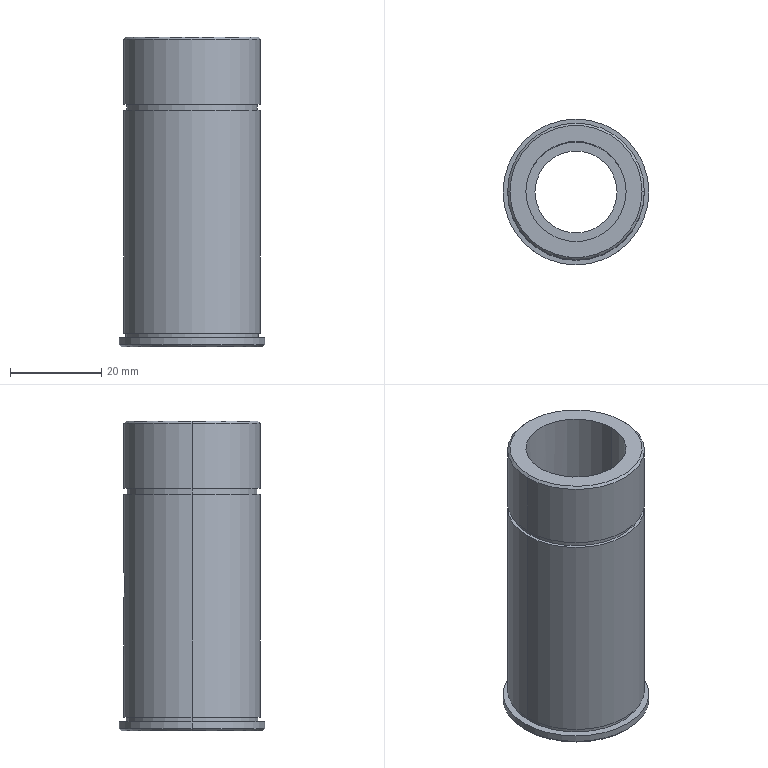Part | SolidWorks | features ICE 4, RevCut 2, Chamfer 1, Extrusion 1 | 1 solid | 27 faces | box 32 x 32 x 68 mm | volume 22395 mm3 | cylinder 16 | plane 7 | cone 4 | commonest cylinder face diameters 30 x4 6 x2 18 x2 22 x2 28.6 x2 29 x2
STEP:
#1=CARTESIAN_POINT('',(-14.5,0.,3.));
#2=VERTEX_POINT('',#1);
#3=CARTESIAN_POINT('',(14.5,0.,3.));
#4=VERTEX_POINT('',#3);
#5=CARTESIAN_POINT('',(0.,0.,3.));
#6=DIRECTION('',(0.,0.,-1.));
#7=DIRECTION('',(-1.,0.,0.));
#8=AXIS2_PLACEMENT_3D('',#5,#6,#7);
#9=CIRCLE('',#8,14.5);
#10=EDGE_CURVE('',#2,#4,#9,.T.);
#11=ORIENTED_EDGE('',*,*,#10,.T.);
#12=CARTESIAN_POINT('',(14.5,0.,2.));
#13=VERTEX_POINT('',#12);
#14=CARTESIAN_POINT('',(14.5,0.,0.));
#15=DIRECTION('',(0.,0.,-1.));
#16=VECTOR('',#15,1000.);
#17=LINE('',#14,#16);
#18=EDGE_CURVE('',#4,#13,#17,.T.);
#19=ORIENTED_EDGE('',*,*,#18,.T.);
#20=CARTESIAN_POINT('',(-14.5,0.,2.));
#21=VERTEX_POINT('',#20);
#22=CARTESIAN_POINT('',(0.,0.,2.));
#23=DIRECTION('',(0.,0.,-1.));
#24=DIRECTION('',(-1.,0.,0.));
#25=AXIS2_PLACEMENT_3D('',#22,#23,#24);
#26=CIRCLE('',#25,14.5);
#27=EDGE_CURVE('',#21,#13,#26,.T.);
#28=ORIENTED_EDGE('',*,*,#27,.F.);
#29=CARTESIAN_POINT('',(-14.5,0.,0.));
#30=DIRECTION('',(0.,0.,-1.));
#31=VECTOR('',#30,1000.);
#32=LINE('',#29,#31);
#33=EDGE_CURVE('',#2,#21,#32,.T.);
#34=ORIENTED_EDGE('',*,*,#33,.F.);
#35=EDGE_LOOP('',(#11,#19,#28,#34));
#36=FACE_OUTER_BOUND('',#35,.T.);
#37=CARTESIAN_POINT('',(0.,0.,0.));
#38=DIRECTION('',(0.,0.,-1.));
#39=DIRECTION('',(-1.,0.,0.));
#40=AXIS2_PLACEMENT_3D('',#37,#38,#39);
#41=CYLINDRICAL_SURFACE('',#40,14.5);
#42=ADVANCED_FACE('',(#36),#41,.T.);
#43=CARTESIAN_POINT('',(14.5,0.,68.));
#44=VERTEX_POINT('',#43);
#45=CARTESIAN_POINT('',(-14.5,0.,68.));
#46=VERTEX_POINT('',#45);
#47=CARTESIAN_POINT('',(0.,0.,68.));
#48=DIRECTION('',(0.,0.,1.));
#49=DIRECTION('',(1.,0.,0.));
#50=AXIS2_PLACEMENT_3D('',#47,#48,#49);
#51=CIRCLE('',#50,14.5);
#52=EDGE_CURVE('',#44,#46,#51,.T.);
#53=ORIENTED_EDGE('',*,*,#52,.F.);
#54=CARTESIAN_POINT('',(15.,0.,67.5));
#55=VERTEX_POINT('',#54);
#56=CARTESIAN_POINT('',(14.5,0.,68.));
#57=DIRECTION('',(0.7071,0.,-0.7071));
#58=VECTOR('',#57,1000.);
#59=LINE('',#56,#58);
#60=EDGE_CURVE('',#44,#55,#59,.T.);
#61=ORIENTED_EDGE('',*,*,#60,.T.);
#62=CARTESIAN_POINT('',(-15.,0.,67.5));
#63=VERTEX_POINT('',#62);
#64=CARTESIAN_POINT('',(0.,0.,67.5));
#65=DIRECTION('',(0.,0.,-1.));
#66=DIRECTION('',(1.,0.,0.));
#67=AXIS2_PLACEMENT_3D('',#64,#65,#66);
#68=CIRCLE('',#67,15.);
#69=EDGE_CURVE('',#63,#55,#68,.T.);
#70=ORIENTED_EDGE('',*,*,#69,.F.);
#71=CARTESIAN_POINT('',(-14.5,0.,68.));
#72=DIRECTION('',(-0.7071,0.,-0.7071));
#73=VECTOR('',#72,1000.);
#74=LINE('',#71,#73);
#75=EDGE_CURVE('',#46,#63,#74,.T.);
#76=ORIENTED_EDGE('',*,*,#75,.F.);
#77=EDGE_LOOP('',(#53,#61,#70,#76));
#78=FACE_OUTER_BOUND('',#77,.T.);
#79=CARTESIAN_POINT('',(0.,0.,68.));
#80=DIRECTION('',(0.,0.,-1.));
#81=DIRECTION('',(-1.,0.,0.));
#82=AXIS2_PLACEMENT_3D('',#79,#80,#81);
#83=CONICAL_SURFACE('',#82,14.5,0.7854);
#84=ADVANCED_FACE('',(#78),#83,.T.);
#85=CARTESIAN_POINT('',(-15.5,0.,0.));
#86=VERTEX_POINT('',#85);
#87=CARTESIAN_POINT('',(15.5,0.,0.));
#88=VERTEX_POINT('',#87);
#89=CARTESIAN_POINT('',(0.,0.,0.));
#90=DIRECTION('',(0.,0.,-1.));
#91=DIRECTION('',(1.,0.,0.));
#92=AXIS2_PLACEMENT_3D('',#89,#90,#91);
#93=CIRCLE('',#92,15.5);
#94=EDGE_CURVE('',#86,#88,#93,.T.);
#95=ORIENTED_EDGE('',*,*,#94,.F.);
#96=CARTESIAN_POINT('',(-16.,0.,0.5));
#97=VERTEX_POINT('',#96);
#98=CARTESIAN_POINT('',(-16.,0.,0.5));
#99=DIRECTION('',(-0.7071,0.,0.7071));
#100=VECTOR('',#99,1000.);
#101=LINE('',#98,#100);
#102=EDGE_CURVE('',#86,#97,#101,.T.);
#103=ORIENTED_EDGE('',*,*,#102,.T.);
#104=CARTESIAN_POINT('',(16.,0.,0.5));
#105=VERTEX_POINT('',#104);
#106=CARTESIAN_POINT('',(0.,0.,0.5));
#107=DIRECTION('',(0.,0.,1.));
#108=DIRECTION('',(1.,0.,0.));
#109=AXIS2_PLACEMENT_3D('',#106,#107,#108);
#110=CIRCLE('',#109,16.);
#111=EDGE_CURVE('',#105,#97,#110,.T.);
#112=ORIENTED_EDGE('',*,*,#111,.F.);
#113=CARTESIAN_POINT('',(16.,0.,0.5));
#114=DIRECTION('',(0.7071,0.,0.7071));
#115=VECTOR('',#114,1000.);
#116=LINE('',#113,#115);
#117=EDGE_CURVE('',#88,#105,#116,.T.);
#118=ORIENTED_EDGE('',*,*,#117,.F.);
#119=EDGE_LOOP('',(#95,#103,#112,#118));
#120=FACE_OUTER_BOUND('',#119,.T.);
#121=CARTESIAN_POINT('',(0.,0.,0.5));
#122=DIRECTION('',(0.,0.,1.));
#123=DIRECTION('',(1.,0.,0.));
#124=AXIS2_PLACEMENT_3D('',#121,#122,#123);
#125=CONICAL_SURFACE('',#124,16.,0.7854);
#126=ADVANCED_FACE('',(#120),#125,.T.);
#127=CARTESIAN_POINT('',(14.3,0.,51.9));
#128=VERTEX_POINT('',#127);
#129=CARTESIAN_POINT('',(-14.3,0.,51.9));
#130=VERTEX_POINT('',#129);
#131=CARTESIAN_POINT('',(0.,0.,51.9));
#132=DIRECTION('',(0.,0.,1.));
#133=DIRECTION('',(1.,0.,0.));
#134=AXIS2_PLACEMENT_3D('',#131,#132,#133);
#135=CIRCLE('',#134,14.3);
#136=EDGE_CURVE('',#128,#130,#135,.T.);
#137=ORIENTED_EDGE('',*,*,#136,.T.);
#138=CARTESIAN_POINT('',(-14.3,0.,53.2));
#139=VERTEX_POINT('',#138);
#140=CARTESIAN_POINT('',(-14.3,0.,68.));
#141=DIRECTION('',(0.,0.,1.));
#142=VECTOR('',#141,1000.);
#143=LINE('',#140,#142);
#144=EDGE_CURVE('',#130,#139,#143,.T.);
#145=ORIENTED_EDGE('',*,*,#144,.T.);
#146=CARTESIAN_POINT('',(14.3,0.,53.2));
#147=VERTEX_POINT('',#146);
#148=CARTESIAN_POINT('',(0.,0.,53.2));
#149=DIRECTION('',(0.,0.,1.));
#150=DIRECTION('',(1.,0.,0.));
#151=AXIS2_PLACEMENT_3D('',#148,#149,#150);
#152=CIRCLE('',#151,14.3);
#153=EDGE_CURVE('',#147,#139,#152,.T.);
#154=ORIENTED_EDGE('',*,*,#153,.F.);
#155=CARTESIAN_POINT('',(14.3,0.,68.));
#156=DIRECTION('',(0.,0.,1.));
#157=VECTOR('',#156,1000.);
#158=LINE('',#155,#157);
#159=EDGE_CURVE('',#128,#147,#158,.T.);
#160=ORIENTED_EDGE('',*,*,#159,.F.);
#161=EDGE_LOOP('',(#137,#145,#154,#160));
#162=FACE_OUTER_BOUND('',#161,.T.);
#163=CARTESIAN_POINT('',(0.,0.,68.));
#164=DIRECTION('',(0.,0.,1.));
#165=DIRECTION('',(1.,0.,0.));
#166=AXIS2_PLACEMENT_3D('',#163,#164,#165);
#167=CYLINDRICAL_SURFACE('',#166,14.3);
#168=ADVANCED_FACE('',(#162),#167,.T.);
#169=CARTESIAN_POINT('',(0.,11.,29.));
#170=VERTEX_POINT('',#169);
#171=CARTESIAN_POINT('',(0.,11.,35.));
#172=VERTEX_POINT('',#171);
#173=CARTESIAN_POINT('',(0.,11.,29.));
#174=CARTESIAN_POINT('',(-0.3926,11.,29.));
#175=CARTESIAN_POINT('',(-0.7891,10.978,29.079));
#176=CARTESIAN_POINT('',(-1.331,10.921,29.304));
#177=CARTESIAN_POINT('',(-1.507,10.898,29.399));
#178=CARTESIAN_POINT('',(-1.832,10.848,29.616));
#179=CARTESIAN_POINT('',(-1.982,10.821,29.74));
#180=CARTESIAN_POINT('',(-2.259,10.766,30.016));
#181=CARTESIAN_POINT('',(-2.385,10.739,30.17));
#182=CARTESIAN_POINT('',(-2.601,10.689,30.493));
#183=CARTESIAN_POINT('',(-2.694,10.665,30.665));
#184=CARTESIAN_POINT('',(-2.846,10.626,31.031));
#185=CARTESIAN_POINT('',(-2.903,10.61,31.219));
#186=CARTESIAN_POINT('',(-2.98,10.589,31.603));
#187=CARTESIAN_POINT('',(-3.,10.583,31.802));
#188=CARTESIAN_POINT('',(-3.,10.583,32.197));
#189=CARTESIAN_POINT('',(-2.981,10.589,32.392));
#190=CARTESIAN_POINT('',(-2.904,10.61,32.778));
#191=CARTESIAN_POINT('',(-2.846,10.626,32.97));
#192=CARTESIAN_POINT('',(-2.696,10.665,33.331));
#193=CARTESIAN_POINT('',(-2.603,10.688,33.504));
#194=CARTESIAN_POINT('',(-2.384,10.739,33.831));
#195=CARTESIAN_POINT('',(-2.26,10.766,33.983));
#196=CARTESIAN_POINT('',(-1.985,10.82,34.258));
#197=CARTESIAN_POINT('',(-1.832,10.848,34.383));
#198=CARTESIAN_POINT('',(-1.506,10.898,34.602));
#199=CARTESIAN_POINT('',(-1.334,10.92,34.694));
#200=CARTESIAN_POINT('',(-0.973,10.958,34.845));
#201=CARTESIAN_POINT('',(-0.7816,10.974,34.903));
#202=CARTESIAN_POINT('',(-0.3953,10.995,34.98));
#203=CARTESIAN_POINT('',(-0.1992,11.,35.));
#204=CARTESIAN_POINT('',(0.,11.,35.));
#205=B_SPLINE_CURVE_WITH_KNOTS('',3,(#173,#174,#175,#176,#177,#178,#179,#180,#181,#182,#183,#184,#185,#186,#187,#188,#189,#190,#191,#192,#193,#194,#195,#196,#197,#198,#199,#200,#201,#202,#203,#204),.UNSPECIFIED.,.F.,.F.,(4,2,2,2,2,2,2,2,2,2,2,2,2,2,2,4),(0.009424,0.0106,0.01119,0.01178,0.01237,0.01296,0.01355,0.01414,0.01472,0.01531,0.0159,0.01649,0.01708,0.01767,0.01826,0.01885),.UNSPECIFIED.);
#206=EDGE_CURVE('',#170,#172,#205,.T.);
#207=ORIENTED_EDGE('',*,*,#206,.F.);
#208=CARTESIAN_POINT('',(0.,15.,29.));
#209=VERTEX_POINT('',#208);
#210=CARTESIAN_POINT('',(0.,5.,29.));
#211=DIRECTION('',(0.,1.,0.));
#212=VECTOR('',#211,1000.);
#213=LINE('',#210,#212);
#214=EDGE_CURVE('',#170,#209,#213,.T.);
#215=ORIENTED_EDGE('',*,*,#214,.T.);
#216=CARTESIAN_POINT('',(0.,15.,35.));
#217=VERTEX_POINT('',#216);
#218=CARTESIAN_POINT('',(0.,15.,35.));
#219=CARTESIAN_POINT('',(-0.1988,15.,35.));
#220=CARTESIAN_POINT('',(-0.3941,14.996,34.98));
#221=CARTESIAN_POINT('',(-0.7782,14.981,34.904));
#222=CARTESIAN_POINT('',(-0.9691,14.97,34.846));
#223=CARTESIAN_POINT('',(-1.332,14.942,34.695));
#224=CARTESIAN_POINT('',(-1.504,14.925,34.603));
#225=CARTESIAN_POINT('',(-1.83,14.889,34.385));
#226=CARTESIAN_POINT('',(-1.984,14.869,34.259));
#227=CARTESIAN_POINT('',(-2.26,14.829,33.983));
#228=CARTESIAN_POINT('',(-2.384,14.81,33.832));
#229=CARTESIAN_POINT('',(-2.603,14.773,33.504));
#230=CARTESIAN_POINT('',(-2.696,14.756,33.33));
#231=CARTESIAN_POINT('',(-2.846,14.728,32.97));
#232=CARTESIAN_POINT('',(-2.904,14.716,32.78));
#233=CARTESIAN_POINT('',(-2.981,14.701,32.392));
#234=CARTESIAN_POINT('',(-3.,14.697,32.197));
#235=CARTESIAN_POINT('',(-3.,14.697,31.805));
#236=CARTESIAN_POINT('',(-2.98,14.701,31.606));
#237=CARTESIAN_POINT('',(-2.904,14.716,31.22));
#238=CARTESIAN_POINT('',(-2.847,14.728,31.033));
#239=CARTESIAN_POINT('',(-2.696,14.756,30.669));
#240=CARTESIAN_POINT('',(-2.602,14.773,30.494));
#241=CARTESIAN_POINT('',(-2.385,14.81,30.17));
#242=CARTESIAN_POINT('',(-2.261,14.829,30.018));
#243=CARTESIAN_POINT('',(-1.982,14.869,29.739));
#244=CARTESIAN_POINT('',(-1.831,14.889,29.615));
#245=CARTESIAN_POINT('',(-1.506,14.925,29.398));
#246=CARTESIAN_POINT('',(-1.331,14.942,29.304));
#247=CARTESIAN_POINT('',(-0.9679,14.97,29.154));
#248=CARTESIAN_POINT('',(-0.7808,14.981,29.097));
#249=CARTESIAN_POINT('',(-0.3952,14.996,29.02));
#250=CARTESIAN_POINT('',(-0.1961,15.,29.));
#251=CARTESIAN_POINT('',(0.,15.,29.));
#252=B_SPLINE_CURVE_WITH_KNOTS('',3,(#218,#219,#220,#221,#222,#223,#224,#225,#226,#227,#228,#229,#230,#231,#232,#233,#234,#235,#236,#237,#238,#239,#240,#241,#242,#243,#244,#245,#246,#247,#248,#249,#250,#251),.UNSPECIFIED.,.F.,.F.,(4,2,2,2,2,2,2,2,2,2,2,2,2,2,2,2,4),(0.,0.0005877,0.001175,0.001763,0.002351,0.002938,0.003526,0.004114,0.004702,0.005289,0.005877,0.006465,0.007052,0.00764,0.008228,0.008815,0.009403),.UNSPECIFIED.);
#253=EDGE_CURVE('',#217,#209,#252,.T.);
#254=ORIENTED_EDGE('',*,*,#253,.F.);
#255=CARTESIAN_POINT('',(0.,5.,35.));
#256=DIRECTION('',(0.,1.,0.));
#257=VECTOR('',#256,1000.);
#258=LINE('',#255,#257);
#259=EDGE_CURVE('',#172,#217,#258,.T.);
#260=ORIENTED_EDGE('',*,*,#259,.F.);
#261=EDGE_LOOP('',(#207,#215,#254,#260));
#262=FACE_OUTER_BOUND('',#261,.T.);
#263=CARTESIAN_POINT('',(0.,5.,32.));
#264=DIRECTION('',(0.,1.,0.));
#265=DIRECTION('',(0.,0.,1.));
#266=AXIS2_PLACEMENT_3D('',#263,#264,#265);
#267=CYLINDRICAL_SURFACE('',#266,3.);
#268=ADVANCED_FACE('',(#262),#267,.F.);
#269=CARTESIAN_POINT('',(-11.,0.,2.));
#270=VERTEX_POINT('',#269);
#271=CARTESIAN_POINT('',(11.,0.,2.));
#272=VERTEX_POINT('',#271);
#273=CARTESIAN_POINT('',(0.,0.,2.));
#274=DIRECTION('',(0.,0.,1.));
#275=DIRECTION('',(1.,0.,0.));
#276=AXIS2_PLACEMENT_3D('',#273,#274,#275);
#277=CIRCLE('',#276,11.);
#278=EDGE_CURVE('',#270,#272,#277,.T.);
#279=ORIENTED_EDGE('',*,*,#278,.F.);
#280=CARTESIAN_POINT('',(-11.,0.,68.));
#281=VERTEX_POINT('',#280);
#282=CARTESIAN_POINT('',(-11.,0.,2.));
#283=DIRECTION('',(0.,0.,1.));
#284=VECTOR('',#283,1000.);
#285=LINE('',#282,#284);
#286=EDGE_CURVE('',#270,#281,#285,.T.);
#287=ORIENTED_EDGE('',*,*,#286,.T.);
#288=CARTESIAN_POINT('',(11.,0.,68.));
#289=VERTEX_POINT('',#288);
#290=CARTESIAN_POINT('',(0.,0.,68.));
#291=DIRECTION('',(0.,0.,1.));
#292=DIRECTION('',(1.,0.,0.));
#293=AXIS2_PLACEMENT_3D('',#290,#291,#292);
#294=CIRCLE('',#293,11.);
#295=EDGE_CURVE('',#281,#289,#294,.T.);
#296=ORIENTED_EDGE('',*,*,#295,.T.);
#297=CARTESIAN_POINT('',(11.,0.,2.));
#298=DIRECTION('',(0.,0.,1.));
#299=VECTOR('',#298,1000.);
#300=LINE('',#297,#299);
#301=EDGE_CURVE('',#272,#289,#300,.T.);
#302=ORIENTED_EDGE('',*,*,#301,.F.);
#303=EDGE_LOOP('',(#279,#287,#296,#302));
#304=FACE_OUTER_BOUND('',#303,.T.);
#305=CARTESIAN_POINT('',(0.,0.,2.));
#306=DIRECTION('',(0.,0.,1.));
#307=DIRECTION('',(1.,0.,0.));
#308=AXIS2_PLACEMENT_3D('',#305,#306,#307);
#309=CYLINDRICAL_SURFACE('',#308,11.);
#310=ADVANCED_FACE('',(#304),#309,.F.);
#311=CARTESIAN_POINT('',(16.,0.,2.));
#312=VERTEX_POINT('',#311);
#313=CARTESIAN_POINT('',(-16.,0.,2.));
#314=VERTEX_POINT('',#313);
#315=CARTESIAN_POINT('',(0.,0.,2.));
#316=DIRECTION('',(0.,0.,1.));
#317=DIRECTION('',(1.,0.,0.));
#318=AXIS2_PLACEMENT_3D('',#315,#316,#317);
#319=CIRCLE('',#318,16.);
#320=EDGE_CURVE('',#312,#314,#319,.T.);
#321=ORIENTED_EDGE('',*,*,#320,.F.);
#322=CARTESIAN_POINT('',(16.,0.,2.));
#323=DIRECTION('',(0.,0.,-1.));
#324=VECTOR('',#323,1000.);
#325=LINE('',#322,#324);
#326=EDGE_CURVE('',#312,#105,#325,.T.);
#327=ORIENTED_EDGE('',*,*,#326,.T.);
#328=ORIENTED_EDGE('',*,*,#111,.T.);
#329=CARTESIAN_POINT('',(-16.,0.,2.));
#330=DIRECTION('',(0.,0.,-1.));
#331=VECTOR('',#330,1000.);
#332=LINE('',#329,#331);
#333=EDGE_CURVE('',#314,#97,#332,.T.);
#334=ORIENTED_EDGE('',*,*,#333,.F.);
#335=EDGE_LOOP('',(#321,#327,#328,#334));
#336=FACE_OUTER_BOUND('',#335,.T.);
#337=CARTESIAN_POINT('',(0.,0.,2.));
#338=DIRECTION('',(0.,0.,-1.));
#339=DIRECTION('',(-1.,0.,0.));
#340=AXIS2_PLACEMENT_3D('',#337,#338,#339);
#341=CYLINDRICAL_SURFACE('',#340,16.);
#342=ADVANCED_FACE('',(#336),#341,.T.);
#343=CARTESIAN_POINT('',(9.,0.,2.));
#344=VERTEX_POINT('',#343);
#345=CARTESIAN_POINT('',(-9.,0.,2.));
#346=VERTEX_POINT('',#345);
#347=CARTESIAN_POINT('',(0.,0.,2.));
#348=DIRECTION('',(0.,0.,-1.));
#349=DIRECTION('',(1.,0.,0.));
#350=AXIS2_PLACEMENT_3D('',#347,#348,#349);
#351=CIRCLE('',#350,9.);
#352=EDGE_CURVE('',#344,#346,#351,.T.);
#353=ORIENTED_EDGE('',*,*,#352,.F.);
#354=CARTESIAN_POINT('',(9.,0.,0.));
#355=VERTEX_POINT('',#354);
#356=CARTESIAN_POINT('',(9.,0.,68.));
#357=DIRECTION('',(0.,0.,-1.));
#358=VECTOR('',#357,1000.);
#359=LINE('',#356,#358);
#360=EDGE_CURVE('',#344,#355,#359,.T.);
#361=ORIENTED_EDGE('',*,*,#360,.T.);
#362=CARTESIAN_POINT('',(-9.,0.,0.));
#363=VERTEX_POINT('',#362);
#364=CARTESIAN_POINT('',(0.,0.,0.));
#365=DIRECTION('',(0.,0.,-1.));
#366=DIRECTION('',(-1.,0.,0.));
#367=AXIS2_PLACEMENT_3D('',#364,#365,#366);
#368=CIRCLE('',#367,9.);
#369=EDGE_CURVE('',#355,#363,#368,.T.);
#370=ORIENTED_EDGE('',*,*,#369,.T.);
#371=CARTESIAN_POINT('',(-9.,0.,68.));
#372=DIRECTION('',(0.,0.,-1.));
#373=VECTOR('',#372,1000.);
#374=LINE('',#371,#373);
#375=EDGE_CURVE('',#346,#363,#374,.T.);
#376=ORIENTED_EDGE('',*,*,#375,.F.);
#377=EDGE_LOOP('',(#353,#361,#370,#376));
#378=FACE_OUTER_BOUND('',#377,.T.);
#379=CARTESIAN_POINT('',(0.,0.,68.));
#380=DIRECTION('',(0.,0.,-1.));
#381=DIRECTION('',(-1.,0.,0.));
#382=AXIS2_PLACEMENT_3D('',#379,#380,#381);
#383=CYLINDRICAL_SURFACE('',#382,9.);
#384=ADVANCED_FACE('',(#378),#383,.F.);
#385=ORIENTED_EDGE('',*,*,#69,.T.);
#386=CARTESIAN_POINT('',(15.,0.,53.2));
#387=VERTEX_POINT('',#386);
#388=CARTESIAN_POINT('',(15.,0.,68.));
#389=DIRECTION('',(0.,0.,-1.));
#390=VECTOR('',#389,1000.);
#391=LINE('',#388,#390);
#392=EDGE_CURVE('',#55,#387,#391,.T.);
#393=ORIENTED_EDGE('',*,*,#392,.T.);
#394=CARTESIAN_POINT('',(-15.,0.,53.2));
#395=VERTEX_POINT('',#394);
#396=CARTESIAN_POINT('',(0.,0.,53.2));
#397=DIRECTION('',(0.,0.,1.));
#398=DIRECTION('',(1.,0.,0.));
#399=AXIS2_PLACEMENT_3D('',#396,#397,#398);
#400=CIRCLE('',#399,15.);
#401=EDGE_CURVE('',#387,#395,#400,.T.);
#402=ORIENTED_EDGE('',*,*,#401,.T.);
#403=CARTESIAN_POINT('',(-15.,0.,68.));
#404=DIRECTION('',(0.,0.,-1.));
#405=VECTOR('',#404,1000.);
#406=LINE('',#403,#405);
#407=EDGE_CURVE('',#63,#395,#406,.T.);
#408=ORIENTED_EDGE('',*,*,#407,.F.);
#409=EDGE_LOOP('',(#385,#393,#402,#408));
#410=FACE_OUTER_BOUND('',#409,.T.);
#411=CARTESIAN_POINT('',(0.,0.,68.));
#412=DIRECTION('',(0.,0.,-1.));
#413=DIRECTION('',(-1.,0.,0.));
#414=AXIS2_PLACEMENT_3D('',#411,#412,#413);
#415=CYLINDRICAL_SURFACE('',#414,15.);
#416=ADVANCED_FACE('',(#410),#415,.T.);
#417=ORIENTED_EDGE('',*,*,#253,.T.);
#418=CARTESIAN_POINT('',(0.,15.,29.));
#419=CARTESIAN_POINT('',(0.196,15.,29.));
#420=CARTESIAN_POINT('',(0.3912,14.996,29.019));
#421=CARTESIAN_POINT('',(0.7798,14.981,29.096));
#422=CARTESIAN_POINT('',(0.9683,14.97,29.154));
#423=CARTESIAN_POINT('',(1.329,14.942,29.304));
#424=CARTESIAN_POINT('',(1.505,14.925,29.397));
#425=CARTESIAN_POINT('',(1.831,14.889,29.616));
#426=CARTESIAN_POINT('',(1.982,14.869,29.739));
#427=CARTESIAN_POINT('',(2.258,14.83,30.016));
#428=CARTESIAN_POINT('',(2.385,14.81,30.17));
#429=CARTESIAN_POINT('',(2.602,14.773,30.494));
#430=CARTESIAN_POINT('',(2.694,14.756,30.666));
#431=CARTESIAN_POINT('',(2.846,14.728,31.03));
#432=CARTESIAN_POINT('',(2.903,14.716,31.22));
#433=CARTESIAN_POINT('',(2.98,14.701,31.604));
#434=CARTESIAN_POINT('',(3.,14.697,31.8));
#435=CARTESIAN_POINT('',(3.,14.697,32.197));
#436=CARTESIAN_POINT('',(2.981,14.701,32.392));
#437=CARTESIAN_POINT('',(2.904,14.716,32.776));
#438=CARTESIAN_POINT('',(2.847,14.728,32.967));
#439=CARTESIAN_POINT('',(2.696,14.756,33.33));
#440=CARTESIAN_POINT('',(2.604,14.773,33.502));
#441=CARTESIAN_POINT('',(2.386,14.809,33.829));
#442=CARTESIAN_POINT('',(2.26,14.829,33.982));
#443=CARTESIAN_POINT('',(1.847,14.888,34.396));
#444=CARTESIAN_POINT('',(1.513,14.928,34.62));
#445=CARTESIAN_POINT('',(0.9723,14.97,34.845));
#446=CARTESIAN_POINT('',(0.782,14.981,34.903));
#447=CARTESIAN_POINT('',(0.3948,14.996,34.98));
#448=CARTESIAN_POINT('',(0.1987,15.,35.));
#449=CARTESIAN_POINT('',(0.,15.,35.));
#450=B_SPLINE_CURVE_WITH_KNOTS('',3,(#418,#419,#420,#421,#422,#423,#424,#425,#426,#427,#428,#429,#430,#431,#432,#433,#434,#435,#436,#437,#438,#439,#440,#441,#442,#443,#444,#445,#446,#447,#448,#449),.UNSPECIFIED.,.F.,.F.,(4,2,2,2,2,2,2,2,2,2,2,2,2,2,2,4),(0.009403,0.009991,0.01058,0.01117,0.01175,0.01234,0.01293,0.01352,0.0141,0.01469,0.01528,0.01587,0.01645,0.01763,0.01822,0.0188),.UNSPECIFIED.);
#451=EDGE_CURVE('',#209,#217,#450,.T.);
#452=ORIENTED_EDGE('',*,*,#451,.T.);
#453=EDGE_LOOP('',(#417,#452));
#454=FACE_BOUND('',#453,.T.);
#455=CARTESIAN_POINT('',(15.,0.,51.9));
#456=VERTEX_POINT('',#455);
#457=CARTESIAN_POINT('',(-15.,0.,51.9));
#458=VERTEX_POINT('',#457);
#459=CARTESIAN_POINT('',(0.,0.,51.9));
#460=DIRECTION('',(0.,0.,1.));
#461=DIRECTION('',(1.,0.,0.));
#462=AXIS2_PLACEMENT_3D('',#459,#460,#461);
#463=CIRCLE('',#462,15.);
#464=EDGE_CURVE('',#456,#458,#463,.T.);
#465=ORIENTED_EDGE('',*,*,#464,.F.);
#466=CARTESIAN_POINT('',(15.,0.,3.));
#467=VERTEX_POINT('',#466);
#468=CARTESIAN_POINT('',(15.,0.,68.));
#469=DIRECTION('',(0.,0.,-1.));
#470=VECTOR('',#469,1000.);
#471=LINE('',#468,#470);
#472=EDGE_CURVE('',#456,#467,#471,.T.);
#473=ORIENTED_EDGE('',*,*,#472,.T.);
#474=CARTESIAN_POINT('',(-15.,0.,3.));
#475=VERTEX_POINT('',#474);
#476=CARTESIAN_POINT('',(0.,0.,3.));
#477=DIRECTION('',(0.,0.,-1.));
#478=DIRECTION('',(-1.,0.,0.));
#479=AXIS2_PLACEMENT_3D('',#476,#477,#478);
#480=CIRCLE('',#479,15.);
#481=EDGE_CURVE('',#475,#467,#480,.T.);
#482=ORIENTED_EDGE('',*,*,#481,.F.);
#483=CARTESIAN_POINT('',(-15.,0.,68.));
#484=DIRECTION('',(0.,0.,-1.));
#485=VECTOR('',#484,1000.);
#486=LINE('',#483,#485);
#487=EDGE_CURVE('',#458,#475,#486,.T.);
#488=ORIENTED_EDGE('',*,*,#487,.F.);
#489=EDGE_LOOP('',(#465,#473,#482,#488));
#490=FACE_OUTER_BOUND('',#489,.T.);
#491=CARTESIAN_POINT('',(0.,0.,68.));
#492=DIRECTION('',(0.,0.,-1.));
#493=DIRECTION('',(-1.,0.,0.));
#494=AXIS2_PLACEMENT_3D('',#491,#492,#493);
#495=CYLINDRICAL_SURFACE('',#494,15.);
#496=ADVANCED_FACE('',(#454,#490),#495,.T.);
#497=ORIENTED_EDGE('',*,*,#472,.F.);
#498=CARTESIAN_POINT('',(0.,0.,51.9));
#499=DIRECTION('',(0.,0.,1.));
#500=DIRECTION('',(1.,0.,0.));
#501=AXIS2_PLACEMENT_3D('',#498,#499,#500);
#502=CIRCLE('',#501,15.);
#503=EDGE_CURVE('',#458,#456,#502,.T.);
#504=ORIENTED_EDGE('',*,*,#503,.F.);
#505=ORIENTED_EDGE('',*,*,#487,.T.);
#506=CARTESIAN_POINT('',(0.,0.,3.));
#507=DIRECTION('',(0.,0.,-1.));
#508=DIRECTION('',(-1.,0.,0.));
#509=AXIS2_PLACEMENT_3D('',#506,#507,#508);
#510=CIRCLE('',#509,15.);
#511=EDGE_CURVE('',#467,#475,#510,.T.);
#512=ORIENTED_EDGE('',*,*,#511,.F.);
#513=EDGE_LOOP('',(#497,#504,#505,#512));
#514=FACE_OUTER_BOUND('',#513,.T.);
#515=CARTESIAN_POINT('',(0.,0.,68.));
#516=DIRECTION('',(0.,0.,-1.));
#517=DIRECTION('',(-1.,0.,0.));
#518=AXIS2_PLACEMENT_3D('',#515,#516,#517);
#519=CYLINDRICAL_SURFACE('',#518,15.);
#520=ADVANCED_FACE('',(#514),#519,.T.);
#521=ORIENTED_EDGE('',*,*,#392,.F.);
#522=CARTESIAN_POINT('',(0.,0.,67.5));
#523=DIRECTION('',(0.,0.,-1.));
#524=DIRECTION('',(1.,0.,0.));
#525=AXIS2_PLACEMENT_3D('',#522,#523,#524);
#526=CIRCLE('',#525,15.);
#527=EDGE_CURVE('',#55,#63,#526,.T.);
#528=ORIENTED_EDGE('',*,*,#527,.T.);
#529=ORIENTED_EDGE('',*,*,#407,.T.);
#530=CARTESIAN_POINT('',(0.,0.,53.2));
#531=DIRECTION('',(0.,0.,1.));
#532=DIRECTION('',(1.,0.,0.));
#533=AXIS2_PLACEMENT_3D('',#530,#531,#532);
#534=CIRCLE('',#533,15.);
#535=EDGE_CURVE('',#395,#387,#534,.T.);
#536=ORIENTED_EDGE('',*,*,#535,.T.);
#537=EDGE_LOOP('',(#521,#528,#529,#536));
#538=FACE_OUTER_BOUND('',#537,.T.);
#539=CARTESIAN_POINT('',(0.,0.,68.));
#540=DIRECTION('',(0.,0.,-1.));
#541=DIRECTION('',(-1.,0.,0.));
#542=AXIS2_PLACEMENT_3D('',#539,#540,#541);
#543=CYLINDRICAL_SURFACE('',#542,15.);
#544=ADVANCED_FACE('',(#538),#543,.T.);
#545=ORIENTED_EDGE('',*,*,#360,.F.);
#546=CARTESIAN_POINT('',(0.,0.,2.));
#547=DIRECTION('',(0.,0.,-1.));
#548=DIRECTION('',(1.,0.,0.));
#549=AXIS2_PLACEMENT_3D('',#546,#547,#548);
#550=CIRCLE('',#549,9.);
#551=EDGE_CURVE('',#346,#344,#550,.T.);
#552=ORIENTED_EDGE('',*,*,#551,.F.);
#553=ORIENTED_EDGE('',*,*,#375,.T.);
#554=CARTESIAN_POINT('',(0.,0.,0.));
#555=DIRECTION('',(0.,0.,-1.));
#556=DIRECTION('',(-1.,0.,0.));
#557=AXIS2_PLACEMENT_3D('',#554,#555,#556);
#558=CIRCLE('',#557,9.);
#559=EDGE_CURVE('',#363,#355,#558,.T.);
#560=ORIENTED_EDGE('',*,*,#559,.T.);
#561=EDGE_LOOP('',(#545,#552,#553,#560));
#562=FACE_OUTER_BOUND('',#561,.T.);
#563=CARTESIAN_POINT('',(0.,0.,68.));
#564=DIRECTION('',(0.,0.,-1.));
#565=DIRECTION('',(-1.,0.,0.));
#566=AXIS2_PLACEMENT_3D('',#563,#564,#565);
#567=CYLINDRICAL_SURFACE('',#566,9.);
#568=ADVANCED_FACE('',(#562),#567,.F.);
#569=CARTESIAN_POINT('',(0.,0.,2.));
#570=DIRECTION('',(0.,0.,1.));
#571=DIRECTION('',(1.,0.,0.));
#572=AXIS2_PLACEMENT_3D('',#569,#570,#571);
#573=CIRCLE('',#572,16.);
#574=EDGE_CURVE('',#314,#312,#573,.T.);
#575=ORIENTED_EDGE('',*,*,#574,.T.);
#576=ORIENTED_EDGE('',*,*,#320,.T.);
#577=EDGE_LOOP('',(#575,#576));
#578=FACE_OUTER_BOUND('',#577,.T.);
#579=ORIENTED_EDGE('',*,*,#27,.T.);
#580=CARTESIAN_POINT('',(0.,0.,2.));
#581=DIRECTION('',(0.,0.,-1.));
#582=DIRECTION('',(-1.,0.,0.));
#583=AXIS2_PLACEMENT_3D('',#580,#581,#582);
#584=CIRCLE('',#583,14.5);
#585=EDGE_CURVE('',#13,#21,#584,.T.);
#586=ORIENTED_EDGE('',*,*,#585,.T.);
#587=EDGE_LOOP('',(#579,#586));
#588=FACE_BOUND('',#587,.T.);
#589=CARTESIAN_POINT('',(0.,0.,2.));
#590=DIRECTION('',(0.,0.,1.));
#591=DIRECTION('',(1.,0.,0.));
#592=AXIS2_PLACEMENT_3D('',#589,#590,#591);
#593=PLANE('',#592);
#594=ADVANCED_FACE('',(#578,#588),#593,.T.);
#595=ORIENTED_EDGE('',*,*,#326,.F.);
#596=ORIENTED_EDGE('',*,*,#574,.F.);
#597=ORIENTED_EDGE('',*,*,#333,.T.);
#598=CARTESIAN_POINT('',(0.,0.,0.5));
#599=DIRECTION('',(0.,0.,1.));
#600=DIRECTION('',(1.,0.,0.));
#601=AXIS2_PLACEMENT_3D('',#598,#599,#600);
#602=CIRCLE('',#601,16.);
#603=EDGE_CURVE('',#97,#105,#602,.T.);
#604=ORIENTED_EDGE('',*,*,#603,.T.);
#605=EDGE_LOOP('',(#595,#596,#597,#604));
#606=FACE_OUTER_BOUND('',#605,.T.);
#607=CARTESIAN_POINT('',(0.,0.,2.));
#608=DIRECTION('',(0.,0.,-1.));
#609=DIRECTION('',(-1.,0.,0.));
#610=AXIS2_PLACEMENT_3D('',#607,#608,#609);
#611=CYLINDRICAL_SURFACE('',#610,16.);
#612=ADVANCED_FACE('',(#606),#611,.T.);
#613=CARTESIAN_POINT('',(0.,0.,0.));
#614=DIRECTION('',(0.,0.,-1.));
#615=DIRECTION('',(1.,0.,0.));
#616=AXIS2_PLACEMENT_3D('',#613,#614,#615);
#617=CIRCLE('',#616,15.5);
#618=EDGE_CURVE('',#88,#86,#617,.T.);
#619=ORIENTED_EDGE('',*,*,#618,.T.);
#620=ORIENTED_EDGE('',*,*,#94,.T.);
#621=EDGE_LOOP('',(#619,#620));
#622=FACE_OUTER_BOUND('',#621,.T.);
#623=ORIENTED_EDGE('',*,*,#559,.F.);
#624=ORIENTED_EDGE('',*,*,#369,.F.);
#625=EDGE_LOOP('',(#623,#624));
#626=FACE_BOUND('',#625,.T.);
#627=CARTESIAN_POINT('',(0.,0.,0.));
#628=DIRECTION('',(0.,0.,1.));
#629=DIRECTION('',(1.,0.,0.));
#630=AXIS2_PLACEMENT_3D('',#627,#628,#629);
#631=PLANE('',#630);
#632=ADVANCED_FACE('',(#622,#626),#631,.F.);
#633=CARTESIAN_POINT('',(0.,0.,68.));
#634=DIRECTION('',(0.,0.,1.));
#635=DIRECTION('',(1.,0.,0.));
#636=AXIS2_PLACEMENT_3D('',#633,#634,#635);
#637=CIRCLE('',#636,14.5);
#638=EDGE_CURVE('',#46,#44,#637,.T.);
#639=ORIENTED_EDGE('',*,*,#638,.T.);
#640=ORIENTED_EDGE('',*,*,#52,.T.);
#641=EDGE_LOOP('',(#639,#640));
#642=FACE_OUTER_BOUND('',#641,.T.);
#643=CARTESIAN_POINT('',(0.,0.,68.));
#644=DIRECTION('',(0.,0.,1.));
#645=DIRECTION('',(1.,0.,0.));
#646=AXIS2_PLACEMENT_3D('',#643,#644,#645);
#647=CIRCLE('',#646,11.);
#648=EDGE_CURVE('',#289,#281,#647,.T.);
#649=ORIENTED_EDGE('',*,*,#648,.F.);
#650=ORIENTED_EDGE('',*,*,#295,.F.);
#651=EDGE_LOOP('',(#649,#650));
#652=FACE_BOUND('',#651,.T.);
#653=CARTESIAN_POINT('',(0.,0.,68.));
#654=DIRECTION('',(0.,0.,1.));
#655=DIRECTION('',(1.,0.,0.));
#656=AXIS2_PLACEMENT_3D('',#653,#654,#655);
#657=PLANE('',#656);
#658=ADVANCED_FACE('',(#642,#652),#657,.T.);
#659=CARTESIAN_POINT('',(0.,0.,2.));
#660=DIRECTION('',(0.,0.,1.));
#661=DIRECTION('',(1.,0.,0.));
#662=AXIS2_PLACEMENT_3D('',#659,#660,#661);
#663=CIRCLE('',#662,11.);
#664=EDGE_CURVE('',#272,#270,#663,.T.);
#665=ORIENTED_EDGE('',*,*,#664,.T.);
#666=ORIENTED_EDGE('',*,*,#278,.T.);
#667=EDGE_LOOP('',(#665,#666));
#668=FACE_OUTER_BOUND('',#667,.T.);
#669=ORIENTED_EDGE('',*,*,#551,.T.);
#670=ORIENTED_EDGE('',*,*,#352,.T.);
#671=EDGE_LOOP('',(#669,#670));
#672=FACE_BOUND('',#671,.T.);
#673=CARTESIAN_POINT('',(0.,0.,2.));
#674=DIRECTION('',(0.,0.,1.));
#675=DIRECTION('',(1.,0.,0.));
#676=AXIS2_PLACEMENT_3D('',#673,#674,#675);
#677=PLANE('',#676);
#678=ADVANCED_FACE('',(#668,#672),#677,.T.);
#679=ORIENTED_EDGE('',*,*,#286,.F.);
#680=ORIENTED_EDGE('',*,*,#664,.F.);
#681=ORIENTED_EDGE('',*,*,#301,.T.);
#682=ORIENTED_EDGE('',*,*,#648,.T.);
#683=EDGE_LOOP('',(#679,#680,#681,#682));
#684=FACE_OUTER_BOUND('',#683,.T.);
#685=CARTESIAN_POINT('',(0.,11.,35.));
#686=CARTESIAN_POINT('',(0.1992,11.,35.));
#687=CARTESIAN_POINT('',(0.395,10.995,34.98));
#688=CARTESIAN_POINT('',(0.7797,10.974,34.904));
#689=CARTESIAN_POINT('',(0.9708,10.959,34.845));
#690=CARTESIAN_POINT('',(1.334,10.92,34.694));
#691=CARTESIAN_POINT('',(1.506,10.898,34.602));
#692=CARTESIAN_POINT('',(1.831,10.848,34.384));
#693=CARTESIAN_POINT('',(1.984,10.82,34.258));
#694=CARTESIAN_POINT('',(2.26,10.766,33.983));
#695=CARTESIAN_POINT('',(2.383,10.739,33.832));
#696=CARTESIAN_POINT('',(2.603,10.688,33.505));
#697=CARTESIAN_POINT('',(2.695,10.665,33.332));
#698=CARTESIAN_POINT('',(2.845,10.626,32.971));
#699=CARTESIAN_POINT('',(2.903,10.61,32.781));
#700=CARTESIAN_POINT('',(2.981,10.589,32.393));
#701=CARTESIAN_POINT('',(3.,10.583,32.198));
#702=CARTESIAN_POINT('',(3.,10.583,31.805));
#703=CARTESIAN_POINT('',(2.98,10.589,31.605));
#704=CARTESIAN_POINT('',(2.903,10.61,31.219));
#705=CARTESIAN_POINT('',(2.846,10.626,31.032));
#706=CARTESIAN_POINT('',(2.619,10.685,30.485));
#707=CARTESIAN_POINT('',(2.398,10.739,30.155));
#708=CARTESIAN_POINT('',(1.982,10.821,29.739));
#709=CARTESIAN_POINT('',(1.831,10.848,29.616));
#710=CARTESIAN_POINT('',(1.507,10.897,29.399));
#711=CARTESIAN_POINT('',(1.331,10.921,29.305));
#712=CARTESIAN_POINT('',(0.9695,10.959,29.154));
#713=CARTESIAN_POINT('',(0.7824,10.974,29.097));
#714=CARTESIAN_POINT('',(0.3955,10.995,29.02));
#715=CARTESIAN_POINT('',(0.1964,11.,29.));
#716=CARTESIAN_POINT('',(0.,11.,29.));
#717=B_SPLINE_CURVE_WITH_KNOTS('',3,(#685,#686,#687,#688,#689,#690,#691,#692,#693,#694,#695,#696,#697,#698,#699,#700,#701,#702,#703,#704,#705,#706,#707,#708,#709,#710,#711,#712,#713,#714,#715,#716),.UNSPECIFIED.,.F.,.F.,(4,2,2,2,2,2,2,2,2,2,2,2,2,2,2,4),(0.,0.000589,0.001178,0.001767,0.002356,0.002945,0.003534,0.004123,0.004712,0.005301,0.00589,0.007068,0.007657,0.008246,0.008835,0.009424),.UNSPECIFIED.);
#718=EDGE_CURVE('',#172,#170,#717,.T.);
#719=ORIENTED_EDGE('',*,*,#718,.T.);
#720=ORIENTED_EDGE('',*,*,#206,.T.);
#721=EDGE_LOOP('',(#719,#720));
#722=FACE_BOUND('',#721,.T.);
#723=CARTESIAN_POINT('',(0.,0.,2.));
#724=DIRECTION('',(0.,0.,1.));
#725=DIRECTION('',(1.,0.,0.));
#726=AXIS2_PLACEMENT_3D('',#723,#724,#725);
#727=CYLINDRICAL_SURFACE('',#726,11.);
#728=ADVANCED_FACE('',(#684,#722),#727,.F.);
#729=ORIENTED_EDGE('',*,*,#214,.F.);
#730=ORIENTED_EDGE('',*,*,#718,.F.);
#731=ORIENTED_EDGE('',*,*,#259,.T.);
#732=ORIENTED_EDGE('',*,*,#451,.F.);
#733=EDGE_LOOP('',(#729,#730,#731,#732));
#734=FACE_OUTER_BOUND('',#733,.T.);
#735=CARTESIAN_POINT('',(0.,5.,32.));
#736=DIRECTION('',(0.,1.,0.));
#737=DIRECTION('',(0.,0.,1.));
#738=AXIS2_PLACEMENT_3D('',#735,#736,#737);
#739=CYLINDRICAL_SURFACE('',#738,3.);
#740=ADVANCED_FACE('',(#734),#739,.F.);
#741=ORIENTED_EDGE('',*,*,#503,.T.);
#742=ORIENTED_EDGE('',*,*,#464,.T.);
#743=EDGE_LOOP('',(#741,#742));
#744=FACE_OUTER_BOUND('',#743,.T.);
#745=ORIENTED_EDGE('',*,*,#136,.F.);
#746=CARTESIAN_POINT('',(0.,0.,51.9));
#747=DIRECTION('',(0.,0.,1.));
#748=DIRECTION('',(1.,0.,0.));
#749=AXIS2_PLACEMENT_3D('',#746,#747,#748);
#750=CIRCLE('',#749,14.3);
#751=EDGE_CURVE('',#130,#128,#750,.T.);
#752=ORIENTED_EDGE('',*,*,#751,.F.);
#753=EDGE_LOOP('',(#745,#752));
#754=FACE_BOUND('',#753,.T.);
#755=CARTESIAN_POINT('',(0.,15.,51.9));
#756=DIRECTION('',(0.,0.,1.));
#757=DIRECTION('',(1.,0.,0.));
#758=AXIS2_PLACEMENT_3D('',#755,#756,#757);
#759=PLANE('',#758);
#760=ADVANCED_FACE('',(#744,#754),#759,.T.);
#761=ORIENTED_EDGE('',*,*,#144,.F.);
#762=ORIENTED_EDGE('',*,*,#751,.T.);
#763=ORIENTED_EDGE('',*,*,#159,.T.);
#764=CARTESIAN_POINT('',(0.,0.,53.2));
#765=DIRECTION('',(0.,0.,1.));
#766=DIRECTION('',(1.,0.,0.));
#767=AXIS2_PLACEMENT_3D('',#764,#765,#766);
#768=CIRCLE('',#767,14.3);
#769=EDGE_CURVE('',#139,#147,#768,.T.);
#770=ORIENTED_EDGE('',*,*,#769,.F.);
#771=EDGE_LOOP('',(#761,#762,#763,#770));
#772=FACE_OUTER_BOUND('',#771,.T.);
#773=CARTESIAN_POINT('',(0.,0.,68.));
#774=DIRECTION('',(0.,0.,1.));
#775=DIRECTION('',(1.,0.,0.));
#776=AXIS2_PLACEMENT_3D('',#773,#774,#775);
#777=CYLINDRICAL_SURFACE('',#776,14.3);
#778=ADVANCED_FACE('',(#772),#777,.T.);
#779=ORIENTED_EDGE('',*,*,#153,.T.);
#780=ORIENTED_EDGE('',*,*,#769,.T.);
#781=EDGE_LOOP('',(#779,#780));
#782=FACE_BOUND('',#781,.T.);
#783=ORIENTED_EDGE('',*,*,#535,.F.);
#784=ORIENTED_EDGE('',*,*,#401,.F.);
#785=EDGE_LOOP('',(#783,#784));
#786=FACE_OUTER_BOUND('',#785,.T.);
#787=CARTESIAN_POINT('',(0.,15.,53.2));
#788=DIRECTION('',(0.,0.,-1.));
#789=DIRECTION('',(-1.,0.,0.));
#790=AXIS2_PLACEMENT_3D('',#787,#788,#789);
#791=PLANE('',#790);
#792=ADVANCED_FACE('',(#782,#786),#791,.T.);
#793=ORIENTED_EDGE('',*,*,#102,.F.);
#794=ORIENTED_EDGE('',*,*,#618,.F.);
#795=ORIENTED_EDGE('',*,*,#117,.T.);
#796=ORIENTED_EDGE('',*,*,#603,.F.);
#797=EDGE_LOOP('',(#793,#794,#795,#796));
#798=FACE_OUTER_BOUND('',#797,.T.);
#799=CARTESIAN_POINT('',(0.,0.,0.5));
#800=DIRECTION('',(0.,0.,1.));
#801=DIRECTION('',(1.,0.,0.));
#802=AXIS2_PLACEMENT_3D('',#799,#800,#801);
#803=CONICAL_SURFACE('',#802,16.,0.7854);
#804=ADVANCED_FACE('',(#798),#803,.T.);
#805=ORIENTED_EDGE('',*,*,#60,.F.);
#806=ORIENTED_EDGE('',*,*,#638,.F.);
#807=ORIENTED_EDGE('',*,*,#75,.T.);
#808=ORIENTED_EDGE('',*,*,#527,.F.);
#809=EDGE_LOOP('',(#805,#806,#807,#808));
#810=FACE_OUTER_BOUND('',#809,.T.);
#811=CARTESIAN_POINT('',(0.,0.,68.));
#812=DIRECTION('',(0.,0.,-1.));
#813=DIRECTION('',(-1.,0.,0.));
#814=AXIS2_PLACEMENT_3D('',#811,#812,#813);
#815=CONICAL_SURFACE('',#814,14.5,0.7854);
#816=ADVANCED_FACE('',(#810),#815,.T.);
#817=ORIENTED_EDGE('',*,*,#10,.F.);
#818=CARTESIAN_POINT('',(0.,0.,3.));
#819=DIRECTION('',(0.,0.,-1.));
#820=DIRECTION('',(-1.,0.,0.));
#821=AXIS2_PLACEMENT_3D('',#818,#819,#820);
#822=CIRCLE('',#821,14.5);
#823=EDGE_CURVE('',#4,#2,#822,.T.);
#824=ORIENTED_EDGE('',*,*,#823,.F.);
#825=EDGE_LOOP('',(#817,#824));
#826=FACE_BOUND('',#825,.T.);
#827=ORIENTED_EDGE('',*,*,#481,.T.);
#828=ORIENTED_EDGE('',*,*,#511,.T.);
#829=EDGE_LOOP('',(#827,#828));
#830=FACE_OUTER_BOUND('',#829,.T.);
#831=CARTESIAN_POINT('',(-15.,0.,3.));
#832=DIRECTION('',(0.,0.,1.));
#833=DIRECTION('',(1.,0.,0.));
#834=AXIS2_PLACEMENT_3D('',#831,#832,#833);
#835=PLANE('',#834);
#836=ADVANCED_FACE('',(#826,#830),#835,.F.);
#837=ORIENTED_EDGE('',*,*,#18,.F.);
#838=ORIENTED_EDGE('',*,*,#823,.T.);
#839=ORIENTED_EDGE('',*,*,#33,.T.);
#840=ORIENTED_EDGE('',*,*,#585,.F.);
#841=EDGE_LOOP('',(#837,#838,#839,#840));
#842=FACE_OUTER_BOUND('',#841,.T.);
#843=CARTESIAN_POINT('',(0.,0.,0.));
#844=DIRECTION('',(0.,0.,-1.));
#845=DIRECTION('',(-1.,0.,0.));
#846=AXIS2_PLACEMENT_3D('',#843,#844,#845);
#847=CYLINDRICAL_SURFACE('',#846,14.5);
#848=ADVANCED_FACE('',(#842),#847,.T.);
#849=CLOSED_SHELL('',(#42,#84,#126,#168,#268,#310,#342,#384,#416,#496,#520,#544,#568,#594,#612,#632,#658,#678,#728,#740,#760,#778,#792,#804,#816,#836,#848));
#850=MANIFOLD_SOLID_BREP('',#849);
#851=CARTESIAN_POINT('',(0.,0.,0.));
#852=DIRECTION('',(0.,0.,1.));
#853=DIRECTION('',(1.,0.,0.));
#854=AXIS2_PLACEMENT_3D('',#851,#852,#853);
#855=(LENGTH_UNIT()NAMED_UNIT(*)SI_UNIT(.MILLI.,.METRE.));
#856=UNCERTAINTY_MEASURE_WITH_UNIT(LENGTH_MEASURE(0.00001),#855,'','');
#857=(NAMED_UNIT(*)PLANE_ANGLE_UNIT()SI_UNIT($,.RADIAN.));
#858=(NAMED_UNIT(*)SI_UNIT($,.STERADIAN.)SOLID_ANGLE_UNIT());
#859=(GEOMETRIC_REPRESENTATION_CONTEXT(3)GLOBAL_UNCERTAINTY_ASSIGNED_CONTEXT((#856))GLOBAL_UNIT_ASSIGNED_CONTEXT((#855,#857,#858))REPRESENTATION_CONTEXT('',''));
#860=ADVANCED_BREP_SHAPE_REPRESENTATION('',(#850,#854),#859);